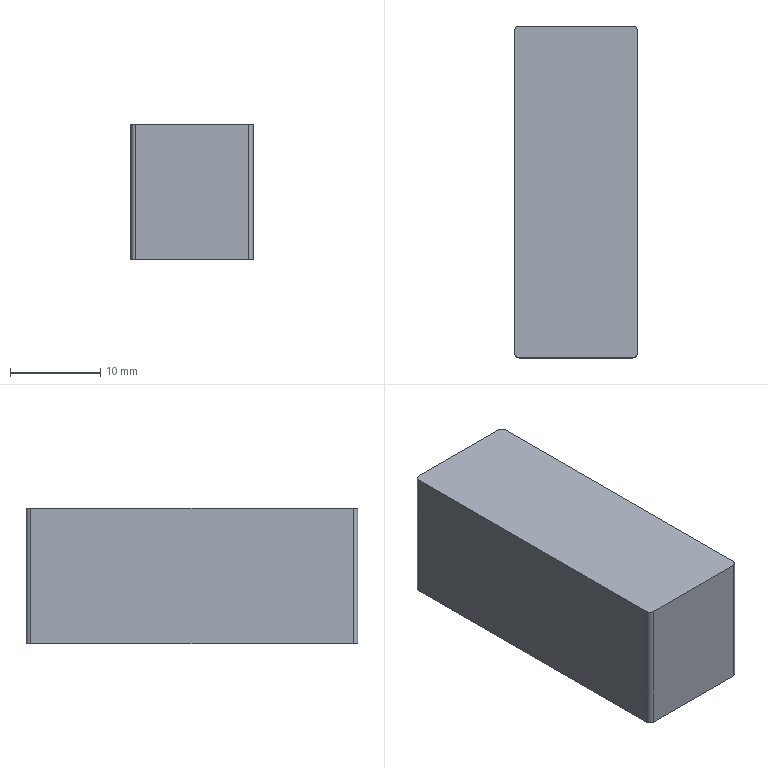Part | NX | features BREP 1 | 1 solid | 10 faces | box 13.542 x 36.72 x 15 mm | volume 7456 mm3 | plane 6 | cylinder 4 | commonest cylinder face diameters 1 x4
STEP:
#1=CARTESIAN_POINT('',(-6.271,18.36,-25.6));
#2=VERTEX_POINT('',#1);
#3=CARTESIAN_POINT('',(-6.771,17.86,-25.6));
#4=VERTEX_POINT('',#3);
#5=CARTESIAN_POINT('',(-6.271,17.86,-25.6));
#6=DIRECTION('',(0.,0.,1.));
#7=DIRECTION('',(1.,0.,0.));
#8=AXIS2_PLACEMENT_3D('',#5,#6,#7);
#9=CIRCLE('',#8,0.5);
#10=EDGE_CURVE('',#2,#4,#9,.T.);
#11=ORIENTED_EDGE('',*,*,#10,.F.);
#12=CARTESIAN_POINT('',(-6.271,18.36,-40.6));
#13=VERTEX_POINT('',#12);
#14=CARTESIAN_POINT('',(-6.271,18.36,-40.6));
#15=DIRECTION('',(0.,0.,1.));
#16=VECTOR('',#15,1000.);
#17=LINE('',#14,#16);
#18=EDGE_CURVE('',#13,#2,#17,.T.);
#19=ORIENTED_EDGE('',*,*,#18,.F.);
#20=CARTESIAN_POINT('',(-6.771,17.86,-40.6));
#21=VERTEX_POINT('',#20);
#22=CARTESIAN_POINT('',(-6.271,17.86,-40.6));
#23=DIRECTION('',(0.,0.,1.));
#24=DIRECTION('',(1.,0.,0.));
#25=AXIS2_PLACEMENT_3D('',#22,#23,#24);
#26=CIRCLE('',#25,0.5);
#27=EDGE_CURVE('',#13,#21,#26,.T.);
#28=ORIENTED_EDGE('',*,*,#27,.T.);
#29=CARTESIAN_POINT('',(-6.771,17.86,-40.6));
#30=DIRECTION('',(0.,0.,1.));
#31=VECTOR('',#30,1000.);
#32=LINE('',#29,#31);
#33=EDGE_CURVE('',#21,#4,#32,.T.);
#34=ORIENTED_EDGE('',*,*,#33,.T.);
#35=EDGE_LOOP('',(#11,#19,#28,#34));
#36=FACE_BOUND('',#35,.T.);
#37=CARTESIAN_POINT('',(-6.271,17.86,-40.6));
#38=DIRECTION('',(0.,0.,1.));
#39=DIRECTION('',(-1.,0.,0.));
#40=AXIS2_PLACEMENT_3D('',#37,#38,#39);
#41=CYLINDRICAL_SURFACE('',#40,0.5);
#42=ADVANCED_FACE('',(#36),#41,.T.);
#43=CARTESIAN_POINT('',(-6.771,-17.86,-25.6));
#44=VERTEX_POINT('',#43);
#45=CARTESIAN_POINT('',(-6.771,-17.86,-25.6));
#46=DIRECTION('',(0.,1.,0.));
#47=VECTOR('',#46,1000.);
#48=LINE('',#45,#47);
#49=EDGE_CURVE('',#44,#4,#48,.T.);
#50=ORIENTED_EDGE('',*,*,#49,.T.);
#51=ORIENTED_EDGE('',*,*,#33,.F.);
#52=CARTESIAN_POINT('',(-6.771,-17.86,-40.6));
#53=VERTEX_POINT('',#52);
#54=CARTESIAN_POINT('',(-6.771,-17.86,-40.6));
#55=DIRECTION('',(0.,1.,0.));
#56=VECTOR('',#55,1000.);
#57=LINE('',#54,#56);
#58=EDGE_CURVE('',#53,#21,#57,.T.);
#59=ORIENTED_EDGE('',*,*,#58,.F.);
#60=CARTESIAN_POINT('',(-6.771,-17.86,-40.6));
#61=DIRECTION('',(0.,0.,1.));
#62=VECTOR('',#61,1000.);
#63=LINE('',#60,#62);
#64=EDGE_CURVE('',#53,#44,#63,.T.);
#65=ORIENTED_EDGE('',*,*,#64,.T.);
#66=EDGE_LOOP('',(#50,#51,#59,#65));
#67=FACE_BOUND('',#66,.T.);
#68=CARTESIAN_POINT('',(-6.771,-17.86,-40.6));
#69=DIRECTION('',(1.,0.,0.));
#70=DIRECTION('',(0.,0.,1.));
#71=AXIS2_PLACEMENT_3D('',#68,#69,#70);
#72=PLANE('',#71);
#73=ADVANCED_FACE('',(#67),#72,.F.);
#74=CARTESIAN_POINT('',(-6.271,-18.36,-25.6));
#75=VERTEX_POINT('',#74);
#76=CARTESIAN_POINT('',(-6.271,-17.86,-25.6));
#77=DIRECTION('',(0.,0.,1.));
#78=DIRECTION('',(1.,0.,0.));
#79=AXIS2_PLACEMENT_3D('',#76,#77,#78);
#80=CIRCLE('',#79,0.5);
#81=EDGE_CURVE('',#44,#75,#80,.T.);
#82=ORIENTED_EDGE('',*,*,#81,.F.);
#83=ORIENTED_EDGE('',*,*,#64,.F.);
#84=CARTESIAN_POINT('',(-6.271,-18.36,-40.6));
#85=VERTEX_POINT('',#84);
#86=CARTESIAN_POINT('',(-6.271,-17.86,-40.6));
#87=DIRECTION('',(0.,0.,1.));
#88=DIRECTION('',(1.,0.,0.));
#89=AXIS2_PLACEMENT_3D('',#86,#87,#88);
#90=CIRCLE('',#89,0.5);
#91=EDGE_CURVE('',#53,#85,#90,.T.);
#92=ORIENTED_EDGE('',*,*,#91,.T.);
#93=CARTESIAN_POINT('',(-6.271,-18.36,-40.6));
#94=DIRECTION('',(0.,0.,1.));
#95=VECTOR('',#94,1000.);
#96=LINE('',#93,#95);
#97=EDGE_CURVE('',#85,#75,#96,.T.);
#98=ORIENTED_EDGE('',*,*,#97,.T.);
#99=EDGE_LOOP('',(#82,#83,#92,#98));
#100=FACE_BOUND('',#99,.T.);
#101=CARTESIAN_POINT('',(-6.271,-17.86,-40.6));
#102=DIRECTION('',(0.,0.,1.));
#103=DIRECTION('',(-1.,0.,0.));
#104=AXIS2_PLACEMENT_3D('',#101,#102,#103);
#105=CYLINDRICAL_SURFACE('',#104,0.5);
#106=ADVANCED_FACE('',(#100),#105,.T.);
#107=CARTESIAN_POINT('',(6.271,-18.36,-25.6));
#108=VERTEX_POINT('',#107);
#109=CARTESIAN_POINT('',(6.271,-18.36,-25.6));
#110=DIRECTION('',(-1.,0.,0.));
#111=VECTOR('',#110,1000.);
#112=LINE('',#109,#111);
#113=EDGE_CURVE('',#108,#75,#112,.T.);
#114=ORIENTED_EDGE('',*,*,#113,.T.);
#115=ORIENTED_EDGE('',*,*,#97,.F.);
#116=CARTESIAN_POINT('',(6.271,-18.36,-40.6));
#117=VERTEX_POINT('',#116);
#118=CARTESIAN_POINT('',(6.271,-18.36,-40.6));
#119=DIRECTION('',(-1.,0.,0.));
#120=VECTOR('',#119,1000.);
#121=LINE('',#118,#120);
#122=EDGE_CURVE('',#117,#85,#121,.T.);
#123=ORIENTED_EDGE('',*,*,#122,.F.);
#124=CARTESIAN_POINT('',(6.271,-18.36,-40.6));
#125=DIRECTION('',(0.,0.,1.));
#126=VECTOR('',#125,1000.);
#127=LINE('',#124,#126);
#128=EDGE_CURVE('',#117,#108,#127,.T.);
#129=ORIENTED_EDGE('',*,*,#128,.T.);
#130=EDGE_LOOP('',(#114,#115,#123,#129));
#131=FACE_BOUND('',#130,.T.);
#132=CARTESIAN_POINT('',(6.271,-18.36,-40.6));
#133=DIRECTION('',(0.,1.,0.));
#134=DIRECTION('',(0.,0.,-1.));
#135=AXIS2_PLACEMENT_3D('',#132,#133,#134);
#136=PLANE('',#135);
#137=ADVANCED_FACE('',(#131),#136,.F.);
#138=CARTESIAN_POINT('',(6.771,-17.86,-25.6));
#139=VERTEX_POINT('',#138);
#140=CARTESIAN_POINT('',(6.271,-17.86,-25.6));
#141=DIRECTION('',(0.,0.,1.));
#142=DIRECTION('',(1.,0.,0.));
#143=AXIS2_PLACEMENT_3D('',#140,#141,#142);
#144=CIRCLE('',#143,0.5);
#145=EDGE_CURVE('',#108,#139,#144,.T.);
#146=ORIENTED_EDGE('',*,*,#145,.F.);
#147=ORIENTED_EDGE('',*,*,#128,.F.);
#148=CARTESIAN_POINT('',(6.771,-17.86,-40.6));
#149=VERTEX_POINT('',#148);
#150=CARTESIAN_POINT('',(6.271,-17.86,-40.6));
#151=DIRECTION('',(0.,0.,1.));
#152=DIRECTION('',(1.,0.,0.));
#153=AXIS2_PLACEMENT_3D('',#150,#151,#152);
#154=CIRCLE('',#153,0.5);
#155=EDGE_CURVE('',#117,#149,#154,.T.);
#156=ORIENTED_EDGE('',*,*,#155,.T.);
#157=CARTESIAN_POINT('',(6.771,-17.86,-40.6));
#158=DIRECTION('',(0.,0.,1.));
#159=VECTOR('',#158,1000.);
#160=LINE('',#157,#159);
#161=EDGE_CURVE('',#149,#139,#160,.T.);
#162=ORIENTED_EDGE('',*,*,#161,.T.);
#163=EDGE_LOOP('',(#146,#147,#156,#162));
#164=FACE_BOUND('',#163,.T.);
#165=CARTESIAN_POINT('',(6.271,-17.86,-40.6));
#166=DIRECTION('',(0.,0.,1.));
#167=DIRECTION('',(-1.,0.,0.));
#168=AXIS2_PLACEMENT_3D('',#165,#166,#167);
#169=CYLINDRICAL_SURFACE('',#168,0.5);
#170=ADVANCED_FACE('',(#164),#169,.T.);
#171=CARTESIAN_POINT('',(6.771,17.86,-25.6));
#172=VERTEX_POINT('',#171);
#173=CARTESIAN_POINT('',(6.771,17.86,-25.6));
#174=DIRECTION('',(0.,-1.,0.));
#175=VECTOR('',#174,1000.);
#176=LINE('',#173,#175);
#177=EDGE_CURVE('',#172,#139,#176,.T.);
#178=ORIENTED_EDGE('',*,*,#177,.T.);
#179=ORIENTED_EDGE('',*,*,#161,.F.);
#180=CARTESIAN_POINT('',(6.771,17.86,-40.6));
#181=VERTEX_POINT('',#180);
#182=CARTESIAN_POINT('',(6.771,17.86,-40.6));
#183=DIRECTION('',(0.,-1.,0.));
#184=VECTOR('',#183,1000.);
#185=LINE('',#182,#184);
#186=EDGE_CURVE('',#181,#149,#185,.T.);
#187=ORIENTED_EDGE('',*,*,#186,.F.);
#188=CARTESIAN_POINT('',(6.771,17.86,-40.6));
#189=DIRECTION('',(0.,0.,1.));
#190=VECTOR('',#189,1000.);
#191=LINE('',#188,#190);
#192=EDGE_CURVE('',#181,#172,#191,.T.);
#193=ORIENTED_EDGE('',*,*,#192,.T.);
#194=EDGE_LOOP('',(#178,#179,#187,#193));
#195=FACE_BOUND('',#194,.T.);
#196=CARTESIAN_POINT('',(6.771,17.86,-40.6));
#197=DIRECTION('',(-1.,0.,0.));
#198=DIRECTION('',(0.,0.,-1.));
#199=AXIS2_PLACEMENT_3D('',#196,#197,#198);
#200=PLANE('',#199);
#201=ADVANCED_FACE('',(#195),#200,.F.);
#202=CARTESIAN_POINT('',(6.271,18.36,-25.6));
#203=VERTEX_POINT('',#202);
#204=CARTESIAN_POINT('',(6.271,17.86,-25.6));
#205=DIRECTION('',(0.,0.,1.));
#206=DIRECTION('',(1.,0.,0.));
#207=AXIS2_PLACEMENT_3D('',#204,#205,#206);
#208=CIRCLE('',#207,0.5);
#209=EDGE_CURVE('',#172,#203,#208,.T.);
#210=ORIENTED_EDGE('',*,*,#209,.F.);
#211=ORIENTED_EDGE('',*,*,#192,.F.);
#212=CARTESIAN_POINT('',(6.271,18.36,-40.6));
#213=VERTEX_POINT('',#212);
#214=CARTESIAN_POINT('',(6.271,17.86,-40.6));
#215=DIRECTION('',(0.,0.,1.));
#216=DIRECTION('',(1.,0.,0.));
#217=AXIS2_PLACEMENT_3D('',#214,#215,#216);
#218=CIRCLE('',#217,0.5);
#219=EDGE_CURVE('',#181,#213,#218,.T.);
#220=ORIENTED_EDGE('',*,*,#219,.T.);
#221=CARTESIAN_POINT('',(6.271,18.36,-40.6));
#222=DIRECTION('',(0.,0.,1.));
#223=VECTOR('',#222,1000.);
#224=LINE('',#221,#223);
#225=EDGE_CURVE('',#213,#203,#224,.T.);
#226=ORIENTED_EDGE('',*,*,#225,.T.);
#227=EDGE_LOOP('',(#210,#211,#220,#226));
#228=FACE_BOUND('',#227,.T.);
#229=CARTESIAN_POINT('',(6.271,17.86,-40.6));
#230=DIRECTION('',(0.,0.,1.));
#231=DIRECTION('',(-1.,0.,0.));
#232=AXIS2_PLACEMENT_3D('',#229,#230,#231);
#233=CYLINDRICAL_SURFACE('',#232,0.5);
#234=ADVANCED_FACE('',(#228),#233,.T.);
#235=CARTESIAN_POINT('',(-6.271,18.36,-25.6));
#236=DIRECTION('',(1.,0.,0.));
#237=VECTOR('',#236,1000.);
#238=LINE('',#235,#237);
#239=EDGE_CURVE('',#2,#203,#238,.T.);
#240=ORIENTED_EDGE('',*,*,#239,.T.);
#241=ORIENTED_EDGE('',*,*,#225,.F.);
#242=CARTESIAN_POINT('',(-6.271,18.36,-40.6));
#243=DIRECTION('',(1.,0.,0.));
#244=VECTOR('',#243,1000.);
#245=LINE('',#242,#244);
#246=EDGE_CURVE('',#13,#213,#245,.T.);
#247=ORIENTED_EDGE('',*,*,#246,.F.);
#248=ORIENTED_EDGE('',*,*,#18,.T.);
#249=EDGE_LOOP('',(#240,#241,#247,#248));
#250=FACE_BOUND('',#249,.T.);
#251=CARTESIAN_POINT('',(-6.271,18.36,-40.6));
#252=DIRECTION('',(0.,-1.,0.));
#253=DIRECTION('',(-1.,0.,0.));
#254=AXIS2_PLACEMENT_3D('',#251,#252,#253);
#255=PLANE('',#254);
#256=ADVANCED_FACE('',(#250),#255,.F.);
#257=ORIENTED_EDGE('',*,*,#27,.F.);
#258=ORIENTED_EDGE('',*,*,#246,.T.);
#259=ORIENTED_EDGE('',*,*,#219,.F.);
#260=ORIENTED_EDGE('',*,*,#186,.T.);
#261=ORIENTED_EDGE('',*,*,#155,.F.);
#262=ORIENTED_EDGE('',*,*,#122,.T.);
#263=ORIENTED_EDGE('',*,*,#91,.F.);
#264=ORIENTED_EDGE('',*,*,#58,.T.);
#265=EDGE_LOOP('',(#257,#258,#259,#260,#261,#262,#263,#264));
#266=FACE_BOUND('',#265,.T.);
#267=CARTESIAN_POINT('',(-6.271,17.86,-40.6));
#268=DIRECTION('',(0.,0.,1.));
#269=DIRECTION('',(-1.,0.,0.));
#270=AXIS2_PLACEMENT_3D('',#267,#268,#269);
#271=PLANE('',#270);
#272=ADVANCED_FACE('',(#266),#271,.F.);
#273=ORIENTED_EDGE('',*,*,#10,.T.);
#274=ORIENTED_EDGE('',*,*,#49,.F.);
#275=ORIENTED_EDGE('',*,*,#81,.T.);
#276=ORIENTED_EDGE('',*,*,#113,.F.);
#277=ORIENTED_EDGE('',*,*,#145,.T.);
#278=ORIENTED_EDGE('',*,*,#177,.F.);
#279=ORIENTED_EDGE('',*,*,#209,.T.);
#280=ORIENTED_EDGE('',*,*,#239,.F.);
#281=EDGE_LOOP('',(#273,#274,#275,#276,#277,#278,#279,#280));
#282=FACE_BOUND('',#281,.T.);
#283=CARTESIAN_POINT('',(-6.271,17.86,-25.6));
#284=DIRECTION('',(0.,0.,1.));
#285=DIRECTION('',(-1.,0.,0.));
#286=AXIS2_PLACEMENT_3D('',#283,#284,#285);
#287=PLANE('',#286);
#288=ADVANCED_FACE('',(#282),#287,.T.);
#289=CLOSED_SHELL('',(#42,#73,#106,#137,#170,#201,#234,#256,#272,#288));
#290=MANIFOLD_SOLID_BREP('',#289);
#291=(LENGTH_UNIT()NAMED_UNIT(*)SI_UNIT(.MILLI.,.METRE.));
#292=UNCERTAINTY_MEASURE_WITH_UNIT(LENGTH_MEASURE(0.00001),#291,'','');
#293=(NAMED_UNIT(*)PLANE_ANGLE_UNIT()SI_UNIT($,.RADIAN.));
#294=(NAMED_UNIT(*)SI_UNIT($,.STERADIAN.)SOLID_ANGLE_UNIT());
#295=(GEOMETRIC_REPRESENTATION_CONTEXT(3)GLOBAL_UNCERTAINTY_ASSIGNED_CONTEXT((#292))GLOBAL_UNIT_ASSIGNED_CONTEXT((#291,#293,#294))REPRESENTATION_CONTEXT('',''));
#296=ADVANCED_BREP_SHAPE_REPRESENTATION('',(#290),#295);